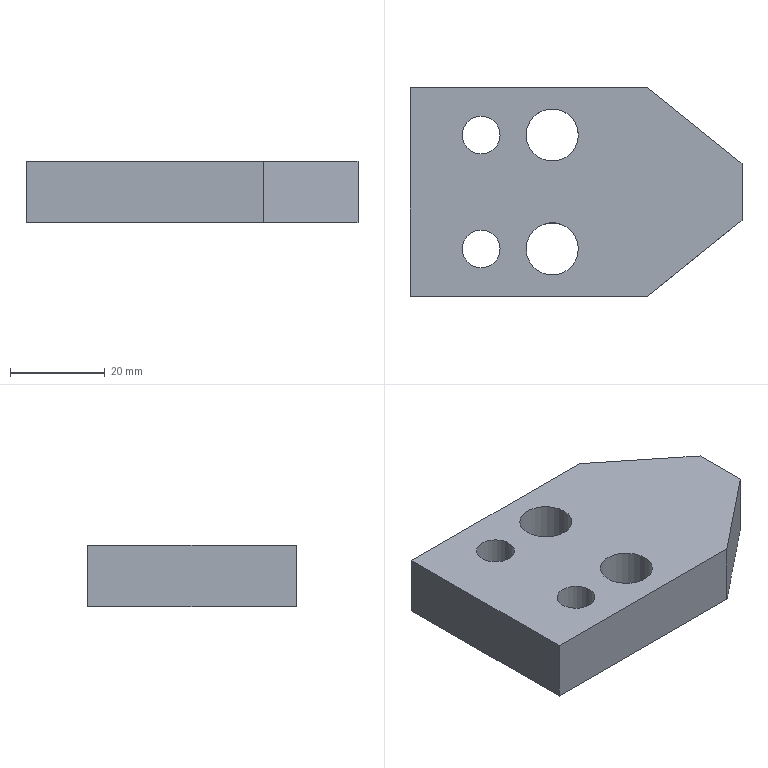Part | NX | features solid 2 | 1 solid | 12 faces | box 70 x 44 x 13 mm | volume 32102 mm3 | plane 8 | cylinder 4 | commonest cylinder face diameters 8 x2 11 x2
STEP:
#1=CARTESIAN_POINT('',(511.818,-101.537,150.));
#2=VERTEX_POINT('',#1);
#3=CARTESIAN_POINT('',(515.818,-101.537,150.));
#4=DIRECTION('',(0.,0.,1.));
#5=DIRECTION('',(-1.,0.,0.));
#6=AXIS2_PLACEMENT_3D('',#3,#4,#5);
#7=CIRCLE('',#6,4.);
#8=EDGE_CURVE('',#2,#2,#7,.T.);
#9=ORIENTED_EDGE('',*,*,#8,.T.);
#10=EDGE_LOOP('',(#9));
#11=FACE_BOUND('',#10,.T.);
#12=CARTESIAN_POINT('',(525.318,-101.537,150.));
#13=VERTEX_POINT('',#12);
#14=CARTESIAN_POINT('',(530.818,-101.537,150.));
#15=DIRECTION('',(0.,0.,1.));
#16=DIRECTION('',(-1.,0.,0.));
#17=AXIS2_PLACEMENT_3D('',#14,#15,#16);
#18=CIRCLE('',#17,5.5);
#19=EDGE_CURVE('',#13,#13,#18,.T.);
#20=ORIENTED_EDGE('',*,*,#19,.T.);
#21=EDGE_LOOP('',(#20));
#22=FACE_BOUND('',#21,.T.);
#23=CARTESIAN_POINT('',(570.818,-119.537,150.));
#24=VERTEX_POINT('',#23);
#25=CARTESIAN_POINT('',(550.818,-135.537,150.));
#26=VERTEX_POINT('',#25);
#27=CARTESIAN_POINT('',(570.818,-119.537,150.));
#28=DIRECTION('',(-0.7809,-0.6247,0.));
#29=VECTOR('',#28,1000.);
#30=LINE('',#27,#29);
#31=EDGE_CURVE('',#24,#26,#30,.T.);
#32=ORIENTED_EDGE('',*,*,#31,.T.);
#33=CARTESIAN_POINT('',(500.818,-135.537,150.));
#34=VERTEX_POINT('',#33);
#35=CARTESIAN_POINT('',(553.818,-135.537,150.));
#36=DIRECTION('',(-1.,0.,0.));
#37=VECTOR('',#36,1000.);
#38=LINE('',#35,#37);
#39=EDGE_CURVE('',#26,#34,#38,.T.);
#40=ORIENTED_EDGE('',*,*,#39,.T.);
#41=CARTESIAN_POINT('',(500.818,-91.537,150.));
#42=VERTEX_POINT('',#41);
#43=CARTESIAN_POINT('',(500.818,-91.537,150.));
#44=DIRECTION('',(0.,-1.,0.));
#45=VECTOR('',#44,1000.);
#46=LINE('',#43,#45);
#47=EDGE_CURVE('',#42,#34,#46,.T.);
#48=ORIENTED_EDGE('',*,*,#47,.F.);
#49=CARTESIAN_POINT('',(550.818,-91.537,150.));
#50=VERTEX_POINT('',#49);
#51=CARTESIAN_POINT('',(553.818,-91.537,150.));
#52=DIRECTION('',(-1.,0.,0.));
#53=VECTOR('',#52,1000.);
#54=LINE('',#51,#53);
#55=EDGE_CURVE('',#50,#42,#54,.T.);
#56=ORIENTED_EDGE('',*,*,#55,.F.);
#57=CARTESIAN_POINT('',(570.818,-107.537,150.));
#58=VERTEX_POINT('',#57);
#59=CARTESIAN_POINT('',(570.818,-107.537,150.));
#60=DIRECTION('',(-0.7809,0.6247,0.));
#61=VECTOR('',#60,1000.);
#62=LINE('',#59,#61);
#63=EDGE_CURVE('',#58,#50,#62,.T.);
#64=ORIENTED_EDGE('',*,*,#63,.F.);
#65=CARTESIAN_POINT('',(570.818,-113.537,150.));
#66=DIRECTION('',(0.,1.,0.));
#67=VECTOR('',#66,1000.);
#68=LINE('',#65,#67);
#69=EDGE_CURVE('',#24,#58,#68,.T.);
#70=ORIENTED_EDGE('',*,*,#69,.F.);
#71=EDGE_LOOP('',(#32,#40,#48,#56,#64,#70));
#72=FACE_BOUND('',#71,.T.);
#73=CARTESIAN_POINT('',(525.318,-125.537,150.));
#74=VERTEX_POINT('',#73);
#75=CARTESIAN_POINT('',(530.818,-125.537,150.));
#76=DIRECTION('',(0.,0.,1.));
#77=DIRECTION('',(-1.,0.,0.));
#78=AXIS2_PLACEMENT_3D('',#75,#76,#77);
#79=CIRCLE('',#78,5.5);
#80=EDGE_CURVE('',#74,#74,#79,.T.);
#81=ORIENTED_EDGE('',*,*,#80,.T.);
#82=EDGE_LOOP('',(#81));
#83=FACE_BOUND('',#82,.T.);
#84=CARTESIAN_POINT('',(511.818,-125.537,150.));
#85=VERTEX_POINT('',#84);
#86=CARTESIAN_POINT('',(515.818,-125.537,150.));
#87=DIRECTION('',(0.,0.,1.));
#88=DIRECTION('',(-1.,0.,0.));
#89=AXIS2_PLACEMENT_3D('',#86,#87,#88);
#90=CIRCLE('',#89,4.);
#91=EDGE_CURVE('',#85,#85,#90,.T.);
#92=ORIENTED_EDGE('',*,*,#91,.T.);
#93=EDGE_LOOP('',(#92));
#94=FACE_BOUND('',#93,.T.);
#95=CARTESIAN_POINT('',(503.818,-91.537,150.));
#96=DIRECTION('',(0.,0.,1.));
#97=DIRECTION('',(1.,0.,0.));
#98=AXIS2_PLACEMENT_3D('',#95,#96,#97);
#99=PLANE('',#98);
#100=ADVANCED_FACE('',(#11,#22,#72,#83,#94),#99,.F.);
#101=CARTESIAN_POINT('',(511.818,-101.537,163.));
#102=VERTEX_POINT('',#101);
#103=CARTESIAN_POINT('',(515.818,-101.537,163.));
#104=DIRECTION('',(0.,0.,1.));
#105=DIRECTION('',(-1.,0.,0.));
#106=AXIS2_PLACEMENT_3D('',#103,#104,#105);
#107=CIRCLE('',#106,4.);
#108=EDGE_CURVE('',#102,#102,#107,.F.);
#109=ORIENTED_EDGE('',*,*,#108,.T.);
#110=EDGE_LOOP('',(#109));
#111=FACE_BOUND('',#110,.T.);
#112=CARTESIAN_POINT('',(525.318,-101.537,163.));
#113=VERTEX_POINT('',#112);
#114=CARTESIAN_POINT('',(530.818,-101.537,163.));
#115=DIRECTION('',(0.,0.,1.));
#116=DIRECTION('',(-1.,0.,0.));
#117=AXIS2_PLACEMENT_3D('',#114,#115,#116);
#118=CIRCLE('',#117,5.5);
#119=EDGE_CURVE('',#113,#113,#118,.F.);
#120=ORIENTED_EDGE('',*,*,#119,.T.);
#121=EDGE_LOOP('',(#120));
#122=FACE_BOUND('',#121,.T.);
#123=CARTESIAN_POINT('',(550.818,-135.537,163.));
#124=VERTEX_POINT('',#123);
#125=CARTESIAN_POINT('',(500.818,-135.537,163.));
#126=VERTEX_POINT('',#125);
#127=CARTESIAN_POINT('',(503.818,-135.537,163.));
#128=DIRECTION('',(-1.,0.,0.));
#129=VECTOR('',#128,1000.);
#130=LINE('',#127,#129);
#131=EDGE_CURVE('',#124,#126,#130,.T.);
#132=ORIENTED_EDGE('',*,*,#131,.F.);
#133=CARTESIAN_POINT('',(570.818,-119.537,163.));
#134=VERTEX_POINT('',#133);
#135=CARTESIAN_POINT('',(543.623,-141.293,163.));
#136=DIRECTION('',(0.7809,0.6247,0.));
#137=VECTOR('',#136,1000.);
#138=LINE('',#135,#137);
#139=EDGE_CURVE('',#124,#134,#138,.T.);
#140=ORIENTED_EDGE('',*,*,#139,.T.);
#141=CARTESIAN_POINT('',(570.818,-107.537,163.));
#142=VERTEX_POINT('',#141);
#143=CARTESIAN_POINT('',(570.818,-91.537,163.));
#144=DIRECTION('',(0.,1.,0.));
#145=VECTOR('',#144,1000.);
#146=LINE('',#143,#145);
#147=EDGE_CURVE('',#134,#142,#146,.T.);
#148=ORIENTED_EDGE('',*,*,#147,.T.);
#149=CARTESIAN_POINT('',(550.818,-91.537,163.));
#150=VERTEX_POINT('',#149);
#151=CARTESIAN_POINT('',(522.159,-68.61,163.));
#152=DIRECTION('',(0.7809,-0.6247,0.));
#153=VECTOR('',#152,1000.);
#154=LINE('',#151,#153);
#155=EDGE_CURVE('',#150,#142,#154,.T.);
#156=ORIENTED_EDGE('',*,*,#155,.F.);
#157=CARTESIAN_POINT('',(500.818,-91.537,163.));
#158=VERTEX_POINT('',#157);
#159=CARTESIAN_POINT('',(503.818,-91.537,163.));
#160=DIRECTION('',(-1.,0.,0.));
#161=VECTOR('',#160,1000.);
#162=LINE('',#159,#161);
#163=EDGE_CURVE('',#150,#158,#162,.T.);
#164=ORIENTED_EDGE('',*,*,#163,.T.);
#165=CARTESIAN_POINT('',(500.818,-91.537,163.));
#166=DIRECTION('',(0.,-1.,0.));
#167=VECTOR('',#166,1000.);
#168=LINE('',#165,#167);
#169=EDGE_CURVE('',#158,#126,#168,.T.);
#170=ORIENTED_EDGE('',*,*,#169,.T.);
#171=EDGE_LOOP('',(#132,#140,#148,#156,#164,#170));
#172=FACE_BOUND('',#171,.T.);
#173=CARTESIAN_POINT('',(525.318,-125.537,163.));
#174=VERTEX_POINT('',#173);
#175=CARTESIAN_POINT('',(530.818,-125.537,163.));
#176=DIRECTION('',(0.,0.,1.));
#177=DIRECTION('',(-1.,0.,0.));
#178=AXIS2_PLACEMENT_3D('',#175,#176,#177);
#179=CIRCLE('',#178,5.5);
#180=EDGE_CURVE('',#174,#174,#179,.F.);
#181=ORIENTED_EDGE('',*,*,#180,.T.);
#182=EDGE_LOOP('',(#181));
#183=FACE_BOUND('',#182,.T.);
#184=CARTESIAN_POINT('',(511.818,-125.537,163.));
#185=VERTEX_POINT('',#184);
#186=CARTESIAN_POINT('',(515.818,-125.537,163.));
#187=DIRECTION('',(0.,0.,1.));
#188=DIRECTION('',(-1.,0.,0.));
#189=AXIS2_PLACEMENT_3D('',#186,#187,#188);
#190=CIRCLE('',#189,4.);
#191=EDGE_CURVE('',#185,#185,#190,.F.);
#192=ORIENTED_EDGE('',*,*,#191,.T.);
#193=EDGE_LOOP('',(#192));
#194=FACE_BOUND('',#193,.T.);
#195=CARTESIAN_POINT('',(503.818,-91.537,163.));
#196=DIRECTION('',(0.,0.,1.));
#197=DIRECTION('',(1.,0.,0.));
#198=AXIS2_PLACEMENT_3D('',#195,#196,#197);
#199=PLANE('',#198);
#200=ADVANCED_FACE('',(#111,#122,#172,#183,#194),#199,.T.);
#201=CARTESIAN_POINT('',(550.818,-135.537,250.));
#202=DIRECTION('',(0.,0.,-1.));
#203=VECTOR('',#202,1000.);
#204=LINE('',#201,#203);
#205=EDGE_CURVE('',#124,#26,#204,.T.);
#206=ORIENTED_EDGE('',*,*,#205,.F.);
#207=ORIENTED_EDGE('',*,*,#131,.T.);
#208=CARTESIAN_POINT('',(500.818,-135.537,150.));
#209=DIRECTION('',(0.,0.,1.));
#210=VECTOR('',#209,1000.);
#211=LINE('',#208,#210);
#212=EDGE_CURVE('',#34,#126,#211,.T.);
#213=ORIENTED_EDGE('',*,*,#212,.F.);
#214=ORIENTED_EDGE('',*,*,#39,.F.);
#215=EDGE_LOOP('',(#206,#207,#213,#214));
#216=FACE_BOUND('',#215,.T.);
#217=CARTESIAN_POINT('',(553.818,-135.537,150.));
#218=DIRECTION('',(0.,1.,0.));
#219=DIRECTION('',(-1.,0.,0.));
#220=AXIS2_PLACEMENT_3D('',#217,#218,#219);
#221=PLANE('',#220);
#222=ADVANCED_FACE('',(#216),#221,.F.);
#223=CARTESIAN_POINT('',(550.818,-91.537,250.));
#224=DIRECTION('',(0.,0.,-1.));
#225=VECTOR('',#224,1000.);
#226=LINE('',#223,#225);
#227=EDGE_CURVE('',#150,#50,#226,.T.);
#228=ORIENTED_EDGE('',*,*,#227,.T.);
#229=ORIENTED_EDGE('',*,*,#55,.T.);
#230=CARTESIAN_POINT('',(500.818,-91.537,150.));
#231=DIRECTION('',(0.,0.,1.));
#232=VECTOR('',#231,1000.);
#233=LINE('',#230,#232);
#234=EDGE_CURVE('',#42,#158,#233,.T.);
#235=ORIENTED_EDGE('',*,*,#234,.T.);
#236=ORIENTED_EDGE('',*,*,#163,.F.);
#237=EDGE_LOOP('',(#228,#229,#235,#236));
#238=FACE_BOUND('',#237,.T.);
#239=CARTESIAN_POINT('',(553.818,-91.537,150.));
#240=DIRECTION('',(0.,1.,0.));
#241=DIRECTION('',(-1.,0.,0.));
#242=AXIS2_PLACEMENT_3D('',#239,#240,#241);
#243=PLANE('',#242);
#244=ADVANCED_FACE('',(#238),#243,.T.);
#245=ORIENTED_EDGE('',*,*,#169,.F.);
#246=ORIENTED_EDGE('',*,*,#234,.F.);
#247=ORIENTED_EDGE('',*,*,#47,.T.);
#248=ORIENTED_EDGE('',*,*,#212,.T.);
#249=EDGE_LOOP('',(#245,#246,#247,#248));
#250=FACE_BOUND('',#249,.T.);
#251=CARTESIAN_POINT('',(500.818,-91.537,150.));
#252=DIRECTION('',(-1.,0.,0.));
#253=DIRECTION('',(0.,-1.,0.));
#254=AXIS2_PLACEMENT_3D('',#251,#252,#253);
#255=PLANE('',#254);
#256=ADVANCED_FACE('',(#250),#255,.T.);
#257=ORIENTED_EDGE('',*,*,#147,.F.);
#258=CARTESIAN_POINT('',(570.818,-119.537,150.));
#259=DIRECTION('',(0.,0.,1.));
#260=VECTOR('',#259,1000.);
#261=LINE('',#258,#260);
#262=EDGE_CURVE('',#24,#134,#261,.T.);
#263=ORIENTED_EDGE('',*,*,#262,.F.);
#264=ORIENTED_EDGE('',*,*,#69,.T.);
#265=CARTESIAN_POINT('',(570.818,-107.537,150.));
#266=DIRECTION('',(0.,0.,1.));
#267=VECTOR('',#266,1000.);
#268=LINE('',#265,#267);
#269=EDGE_CURVE('',#58,#142,#268,.T.);
#270=ORIENTED_EDGE('',*,*,#269,.T.);
#271=EDGE_LOOP('',(#257,#263,#264,#270));
#272=FACE_BOUND('',#271,.T.);
#273=CARTESIAN_POINT('',(570.818,-113.537,150.));
#274=DIRECTION('',(1.,0.,0.));
#275=DIRECTION('',(0.,1.,0.));
#276=AXIS2_PLACEMENT_3D('',#273,#274,#275);
#277=PLANE('',#276);
#278=ADVANCED_FACE('',(#272),#277,.T.);
#279=ORIENTED_EDGE('',*,*,#155,.T.);
#280=ORIENTED_EDGE('',*,*,#269,.F.);
#281=ORIENTED_EDGE('',*,*,#63,.T.);
#282=ORIENTED_EDGE('',*,*,#227,.F.);
#283=EDGE_LOOP('',(#279,#280,#281,#282));
#284=FACE_BOUND('',#283,.T.);
#285=CARTESIAN_POINT('',(570.818,-107.537,250.));
#286=DIRECTION('',(-0.6247,-0.7809,0.));
#287=DIRECTION('',(0.7809,-0.6247,0.));
#288=AXIS2_PLACEMENT_3D('',#285,#286,#287);
#289=PLANE('',#288);
#290=ADVANCED_FACE('',(#284),#289,.F.);
#291=ORIENTED_EDGE('',*,*,#205,.T.);
#292=ORIENTED_EDGE('',*,*,#31,.F.);
#293=ORIENTED_EDGE('',*,*,#262,.T.);
#294=ORIENTED_EDGE('',*,*,#139,.F.);
#295=EDGE_LOOP('',(#291,#292,#293,#294));
#296=FACE_BOUND('',#295,.T.);
#297=CARTESIAN_POINT('',(570.818,-119.537,250.));
#298=DIRECTION('',(0.6247,-0.7809,0.));
#299=DIRECTION('',(0.7809,0.6247,0.));
#300=AXIS2_PLACEMENT_3D('',#297,#298,#299);
#301=PLANE('',#300);
#302=ADVANCED_FACE('',(#296),#301,.T.);
#303=ORIENTED_EDGE('',*,*,#119,.F.);
#304=EDGE_LOOP('',(#303));
#305=FACE_BOUND('',#304,.T.);
#306=ORIENTED_EDGE('',*,*,#19,.F.);
#307=EDGE_LOOP('',(#306));
#308=FACE_BOUND('',#307,.T.);
#309=CARTESIAN_POINT('',(530.818,-101.537,170.));
#310=DIRECTION('',(0.,0.,-1.));
#311=DIRECTION('',(1.,0.,0.));
#312=AXIS2_PLACEMENT_3D('',#309,#310,#311);
#313=CYLINDRICAL_SURFACE('',#312,5.5);
#314=ADVANCED_FACE('',(#305,#308),#313,.F.);
#315=ORIENTED_EDGE('',*,*,#180,.F.);
#316=EDGE_LOOP('',(#315));
#317=FACE_BOUND('',#316,.T.);
#318=ORIENTED_EDGE('',*,*,#80,.F.);
#319=EDGE_LOOP('',(#318));
#320=FACE_BOUND('',#319,.T.);
#321=CARTESIAN_POINT('',(530.818,-125.537,170.));
#322=DIRECTION('',(0.,0.,-1.));
#323=DIRECTION('',(1.,0.,0.));
#324=AXIS2_PLACEMENT_3D('',#321,#322,#323);
#325=CYLINDRICAL_SURFACE('',#324,5.5);
#326=ADVANCED_FACE('',(#317,#320),#325,.F.);
#327=ORIENTED_EDGE('',*,*,#108,.F.);
#328=EDGE_LOOP('',(#327));
#329=FACE_BOUND('',#328,.T.);
#330=ORIENTED_EDGE('',*,*,#8,.F.);
#331=EDGE_LOOP('',(#330));
#332=FACE_BOUND('',#331,.T.);
#333=CARTESIAN_POINT('',(515.818,-101.537,170.));
#334=DIRECTION('',(0.,0.,-1.));
#335=DIRECTION('',(1.,0.,0.));
#336=AXIS2_PLACEMENT_3D('',#333,#334,#335);
#337=CYLINDRICAL_SURFACE('',#336,4.);
#338=ADVANCED_FACE('',(#329,#332),#337,.F.);
#339=ORIENTED_EDGE('',*,*,#191,.F.);
#340=EDGE_LOOP('',(#339));
#341=FACE_BOUND('',#340,.T.);
#342=ORIENTED_EDGE('',*,*,#91,.F.);
#343=EDGE_LOOP('',(#342));
#344=FACE_BOUND('',#343,.T.);
#345=CARTESIAN_POINT('',(515.818,-125.537,170.));
#346=DIRECTION('',(0.,0.,-1.));
#347=DIRECTION('',(1.,0.,0.));
#348=AXIS2_PLACEMENT_3D('',#345,#346,#347);
#349=CYLINDRICAL_SURFACE('',#348,4.);
#350=ADVANCED_FACE('',(#341,#344),#349,.F.);
#351=CLOSED_SHELL('',(#100,#200,#222,#244,#256,#278,#290,#302,#314,#326,#338,#350));
#352=MANIFOLD_SOLID_BREP('',#351);
#353=(LENGTH_UNIT()NAMED_UNIT(*)SI_UNIT(.MILLI.,.METRE.));
#354=UNCERTAINTY_MEASURE_WITH_UNIT(LENGTH_MEASURE(0.00001),#353,'','');
#355=(NAMED_UNIT(*)PLANE_ANGLE_UNIT()SI_UNIT($,.RADIAN.));
#356=(NAMED_UNIT(*)SI_UNIT($,.STERADIAN.)SOLID_ANGLE_UNIT());
#357=(GEOMETRIC_REPRESENTATION_CONTEXT(3)GLOBAL_UNCERTAINTY_ASSIGNED_CONTEXT((#354))GLOBAL_UNIT_ASSIGNED_CONTEXT((#353,#355,#356))REPRESENTATION_CONTEXT('',''));
#358=ADVANCED_BREP_SHAPE_REPRESENTATION('',(#352),#357);